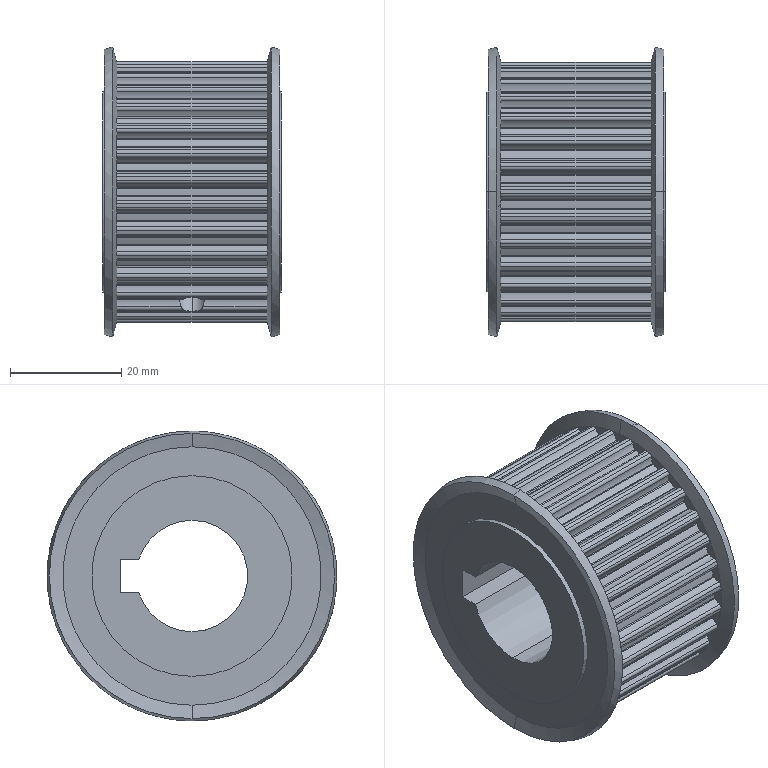Part | STEP file | timing pulley C-HTPA30S5M250-A-N20 | 1 solid | 344 faces | box 32 x 52 x 52 mm | volume 40136 mm3 | cylinder 265 | plane 67 | cone 12 | commonest cylinder face diameters 0.5 x64 1.1 x64 6.55 x64 43.25 x32 46.79 x30 4.917 x4